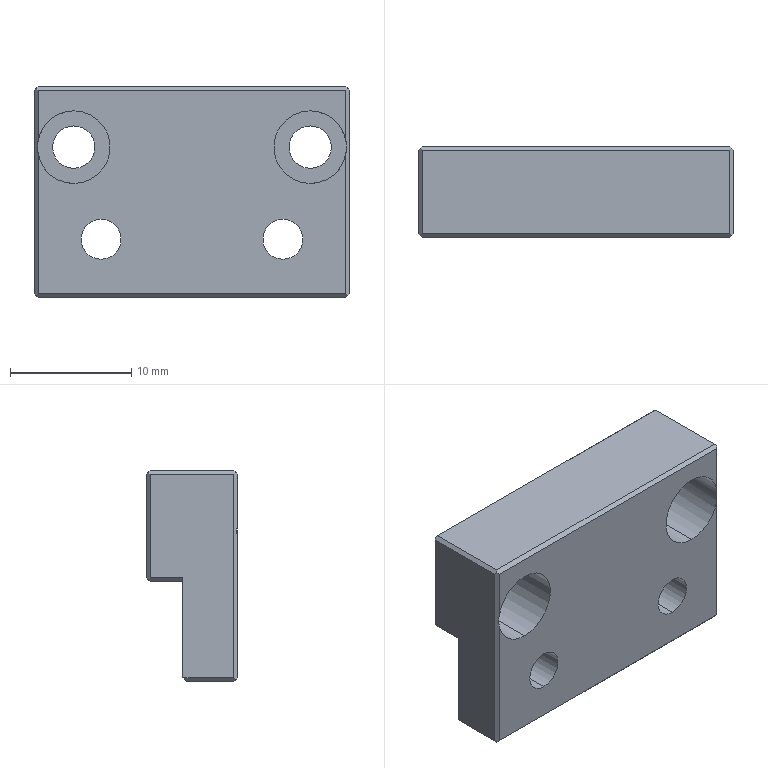Part | NX | 1 solid | 38 faces | box 26 x 7.5 x 17.4 mm | volume 2351 mm3 | plane 26 | cylinder 12 | commonest cylinder face diameters 3.3 x4 3.5 x4 6 x4
STEP:
#1=CARTESIAN_POINT('',(13.59,-63.429,11.253));
#2=VERTEX_POINT('',#1);
#3=CARTESIAN_POINT('',(-11.81,-63.429,11.253));
#4=VERTEX_POINT('',#3);
#5=CARTESIAN_POINT('',(0.8897,-63.429,11.253));
#6=DIRECTION('',(-1.,0.,0.));
#7=VECTOR('',#6,1000.);
#8=LINE('',#5,#7);
#9=EDGE_CURVE('',#2,#4,#8,.T.);
#10=ORIENTED_EDGE('',*,*,#9,.F.);
#11=CARTESIAN_POINT('',(13.59,-66.129,11.253));
#12=VERTEX_POINT('',#11);
#13=CARTESIAN_POINT('',(13.59,-64.629,11.253));
#14=DIRECTION('',(0.,1.,0.));
#15=VECTOR('',#14,1000.);
#16=LINE('',#13,#15);
#17=EDGE_CURVE('',#12,#2,#16,.T.);
#18=ORIENTED_EDGE('',*,*,#17,.F.);
#19=CARTESIAN_POINT('',(-11.81,-66.129,11.253));
#20=VERTEX_POINT('',#19);
#21=CARTESIAN_POINT('',(13.89,-66.129,11.253));
#22=DIRECTION('',(1.,0.,0.));
#23=VECTOR('',#22,1000.);
#24=LINE('',#21,#23);
#25=EDGE_CURVE('',#20,#12,#24,.T.);
#26=ORIENTED_EDGE('',*,*,#25,.F.);
#27=CARTESIAN_POINT('',(-11.81,-64.629,11.253));
#28=DIRECTION('',(0.,-1.,0.));
#29=VECTOR('',#28,1000.);
#30=LINE('',#27,#29);
#31=EDGE_CURVE('',#4,#20,#30,.T.);
#32=ORIENTED_EDGE('',*,*,#31,.F.);
#33=EDGE_LOOP('',(#10,#18,#26,#32));
#34=FACE_BOUND('',#33,.T.);
#35=CARTESIAN_POINT('',(13.89,-66.629,11.253));
#36=DIRECTION('',(0.,0.,-1.));
#37=DIRECTION('',(0.,-1.,0.));
#38=AXIS2_PLACEMENT_3D('',#35,#36,#37);
#39=PLANE('',#38);
#40=ADVANCED_FACE('',(#34),#39,.T.);
#41=CARTESIAN_POINT('',(13.59,-66.129,3.303));
#42=VERTEX_POINT('',#41);
#43=CARTESIAN_POINT('',(-12.11,-66.129,3.303));
#44=VERTEX_POINT('',#43);
#45=CARTESIAN_POINT('',(0.7397,-66.129,3.303));
#46=DIRECTION('',(-1.,0.,0.));
#47=VECTOR('',#46,1000.);
#48=LINE('',#45,#47);
#49=EDGE_CURVE('',#42,#44,#48,.T.);
#50=ORIENTED_EDGE('',*,*,#49,.T.);
#51=CARTESIAN_POINT('',(-12.11,-66.129,11.553));
#52=VERTEX_POINT('',#51);
#53=CARTESIAN_POINT('',(-12.11,-66.129,11.106));
#54=DIRECTION('',(0.,0.,-1.));
#55=VECTOR('',#54,1000.);
#56=LINE('',#53,#55);
#57=EDGE_CURVE('',#52,#44,#56,.T.);
#58=ORIENTED_EDGE('',*,*,#57,.F.);
#59=CARTESIAN_POINT('',(13.89,-66.129,-14.447));
#60=DIRECTION('',(-0.7071,0.,0.7071));
#61=VECTOR('',#60,1000.);
#62=LINE('',#59,#61);
#63=EDGE_CURVE('',#20,#52,#62,.T.);
#64=ORIENTED_EDGE('',*,*,#63,.F.);
#65=ORIENTED_EDGE('',*,*,#25,.T.);
#66=CARTESIAN_POINT('',(13.59,-66.129,11.106));
#67=DIRECTION('',(0.,0.,1.));
#68=VECTOR('',#67,1000.);
#69=LINE('',#66,#68);
#70=EDGE_CURVE('',#42,#12,#69,.T.);
#71=ORIENTED_EDGE('',*,*,#70,.F.);
#72=EDGE_LOOP('',(#50,#58,#64,#65,#71));
#73=FACE_BOUND('',#72,.T.);
#74=CARTESIAN_POINT('',(8.39,-66.129,6.153));
#75=VERTEX_POINT('',#74);
#76=CARTESIAN_POINT('',(8.39,-66.129,9.453));
#77=VERTEX_POINT('',#76);
#78=CARTESIAN_POINT('',(8.39,-66.129,7.803));
#79=DIRECTION('',(0.,-1.,0.));
#80=DIRECTION('',(0.,0.,1.));
#81=AXIS2_PLACEMENT_3D('',#78,#79,#80);
#82=CIRCLE('',#81,1.65);
#83=EDGE_CURVE('',#75,#77,#82,.T.);
#84=ORIENTED_EDGE('',*,*,#83,.T.);
#85=CARTESIAN_POINT('',(8.39,-66.129,7.803));
#86=DIRECTION('',(0.,-1.,0.));
#87=DIRECTION('',(0.,0.,1.));
#88=AXIS2_PLACEMENT_3D('',#85,#86,#87);
#89=CIRCLE('',#88,1.65);
#90=EDGE_CURVE('',#77,#75,#89,.T.);
#91=ORIENTED_EDGE('',*,*,#90,.T.);
#92=EDGE_LOOP('',(#84,#91));
#93=FACE_BOUND('',#92,.T.);
#94=CARTESIAN_POINT('',(-6.61,-66.129,6.153));
#95=VERTEX_POINT('',#94);
#96=CARTESIAN_POINT('',(-6.61,-66.129,9.453));
#97=VERTEX_POINT('',#96);
#98=CARTESIAN_POINT('',(-6.61,-66.129,7.803));
#99=DIRECTION('',(0.,-1.,0.));
#100=DIRECTION('',(0.,0.,1.));
#101=AXIS2_PLACEMENT_3D('',#98,#99,#100);
#102=CIRCLE('',#101,1.65);
#103=EDGE_CURVE('',#95,#97,#102,.T.);
#104=ORIENTED_EDGE('',*,*,#103,.T.);
#105=CARTESIAN_POINT('',(-6.61,-66.129,7.803));
#106=DIRECTION('',(0.,-1.,0.));
#107=DIRECTION('',(0.,0.,1.));
#108=AXIS2_PLACEMENT_3D('',#105,#106,#107);
#109=CIRCLE('',#108,1.65);
#110=EDGE_CURVE('',#97,#95,#109,.T.);
#111=ORIENTED_EDGE('',*,*,#110,.T.);
#112=EDGE_LOOP('',(#104,#111));
#113=FACE_BOUND('',#112,.T.);
#114=CARTESIAN_POINT('',(13.89,-66.129,5.503));
#115=DIRECTION('',(0.,1.,0.));
#116=DIRECTION('',(1.,0.,0.));
#117=AXIS2_PLACEMENT_3D('',#114,#115,#116);
#118=PLANE('',#117);
#119=ADVANCED_FACE('',(#73,#93,#113),#118,.T.);
#120=CARTESIAN_POINT('',(-11.81,-70.329,3.003));
#121=VERTEX_POINT('',#120);
#122=CARTESIAN_POINT('',(-11.81,-66.429,3.003));
#123=VERTEX_POINT('',#122);
#124=CARTESIAN_POINT('',(-11.81,-68.379,3.003));
#125=DIRECTION('',(0.,1.,0.));
#126=VECTOR('',#125,1000.);
#127=LINE('',#124,#126);
#128=EDGE_CURVE('',#121,#123,#127,.T.);
#129=ORIENTED_EDGE('',*,*,#128,.T.);
#130=CARTESIAN_POINT('',(13.59,-66.429,3.003));
#131=VERTEX_POINT('',#130);
#132=CARTESIAN_POINT('',(0.7397,-66.429,3.003));
#133=DIRECTION('',(-1.,0.,0.));
#134=VECTOR('',#133,1000.);
#135=LINE('',#132,#134);
#136=EDGE_CURVE('',#131,#123,#135,.T.);
#137=ORIENTED_EDGE('',*,*,#136,.F.);
#138=CARTESIAN_POINT('',(13.59,-70.329,3.003));
#139=VERTEX_POINT('',#138);
#140=CARTESIAN_POINT('',(13.59,-68.379,3.003));
#141=DIRECTION('',(0.,1.,0.));
#142=VECTOR('',#141,1000.);
#143=LINE('',#140,#142);
#144=EDGE_CURVE('',#139,#131,#143,.T.);
#145=ORIENTED_EDGE('',*,*,#144,.F.);
#146=CARTESIAN_POINT('',(0.7397,-70.329,3.003));
#147=DIRECTION('',(1.,0.,0.));
#148=VECTOR('',#147,1000.);
#149=LINE('',#146,#148);
#150=EDGE_CURVE('',#121,#139,#149,.T.);
#151=ORIENTED_EDGE('',*,*,#150,.F.);
#152=EDGE_LOOP('',(#129,#137,#145,#151));
#153=FACE_BOUND('',#152,.T.);
#154=CARTESIAN_POINT('',(13.89,-70.329,3.003));
#155=DIRECTION('',(0.,0.,-1.));
#156=DIRECTION('',(0.,-1.,0.));
#157=AXIS2_PLACEMENT_3D('',#154,#155,#156);
#158=PLANE('',#157);
#159=ADVANCED_FACE('',(#153),#158,.T.);
#160=CARTESIAN_POINT('',(13.59,-70.629,3.303));
#161=VERTEX_POINT('',#160);
#162=CARTESIAN_POINT('',(13.59,-70.629,14.858));
#163=VERTEX_POINT('',#162);
#164=CARTESIAN_POINT('',(13.59,-70.629,11.106));
#165=DIRECTION('',(0.,0.,1.));
#166=VECTOR('',#165,1000.);
#167=LINE('',#164,#166);
#168=EDGE_CURVE('',#161,#163,#167,.T.);
#169=ORIENTED_EDGE('',*,*,#168,.T.);
#170=CARTESIAN_POINT('',(10.64,-70.629,12.403));
#171=VERTEX_POINT('',#170);
#172=CARTESIAN_POINT('',(10.64,-70.629,15.403));
#173=DIRECTION('',(0.,-1.,0.));
#174=DIRECTION('',(0.,0.,1.));
#175=AXIS2_PLACEMENT_3D('',#172,#173,#174);
#176=CIRCLE('',#175,3.);
#177=EDGE_CURVE('',#171,#163,#176,.T.);
#178=ORIENTED_EDGE('',*,*,#177,.F.);
#179=CARTESIAN_POINT('',(10.64,-70.629,18.403));
#180=VERTEX_POINT('',#179);
#181=CARTESIAN_POINT('',(10.64,-70.629,15.403));
#182=DIRECTION('',(0.,-1.,0.));
#183=DIRECTION('',(0.,0.,1.));
#184=AXIS2_PLACEMENT_3D('',#181,#182,#183);
#185=CIRCLE('',#184,3.);
#186=EDGE_CURVE('',#180,#171,#185,.T.);
#187=ORIENTED_EDGE('',*,*,#186,.F.);
#188=CARTESIAN_POINT('',(13.59,-70.629,15.949));
#189=VERTEX_POINT('',#188);
#190=CARTESIAN_POINT('',(10.64,-70.629,15.403));
#191=DIRECTION('',(0.,-1.,0.));
#192=DIRECTION('',(0.,0.,1.));
#193=AXIS2_PLACEMENT_3D('',#190,#191,#192);
#194=CIRCLE('',#193,3.);
#195=EDGE_CURVE('',#189,#180,#194,.T.);
#196=ORIENTED_EDGE('',*,*,#195,.F.);
#197=CARTESIAN_POINT('',(13.59,-70.629,20.103));
#198=VERTEX_POINT('',#197);
#199=CARTESIAN_POINT('',(13.59,-70.629,11.106));
#200=DIRECTION('',(0.,0.,1.));
#201=VECTOR('',#200,1000.);
#202=LINE('',#199,#201);
#203=EDGE_CURVE('',#189,#198,#202,.T.);
#204=ORIENTED_EDGE('',*,*,#203,.T.);
#205=CARTESIAN_POINT('',(-11.81,-70.629,20.103));
#206=VERTEX_POINT('',#205);
#207=CARTESIAN_POINT('',(0.7397,-70.629,20.103));
#208=DIRECTION('',(-1.,0.,0.));
#209=VECTOR('',#208,1000.);
#210=LINE('',#207,#209);
#211=EDGE_CURVE('',#198,#206,#210,.T.);
#212=ORIENTED_EDGE('',*,*,#211,.T.);
#213=CARTESIAN_POINT('',(-11.81,-70.629,15.949));
#214=VERTEX_POINT('',#213);
#215=CARTESIAN_POINT('',(-11.81,-70.629,11.106));
#216=DIRECTION('',(0.,0.,-1.));
#217=VECTOR('',#216,1000.);
#218=LINE('',#215,#217);
#219=EDGE_CURVE('',#206,#214,#218,.T.);
#220=ORIENTED_EDGE('',*,*,#219,.T.);
#221=CARTESIAN_POINT('',(-8.86,-70.629,18.403));
#222=VERTEX_POINT('',#221);
#223=CARTESIAN_POINT('',(-8.86,-70.629,15.403));
#224=DIRECTION('',(0.,-1.,0.));
#225=DIRECTION('',(0.,0.,1.));
#226=AXIS2_PLACEMENT_3D('',#223,#224,#225);
#227=CIRCLE('',#226,3.);
#228=EDGE_CURVE('',#222,#214,#227,.T.);
#229=ORIENTED_EDGE('',*,*,#228,.F.);
#230=CARTESIAN_POINT('',(-8.86,-70.629,12.403));
#231=VERTEX_POINT('',#230);
#232=CARTESIAN_POINT('',(-8.86,-70.629,15.403));
#233=DIRECTION('',(0.,-1.,0.));
#234=DIRECTION('',(0.,0.,1.));
#235=AXIS2_PLACEMENT_3D('',#232,#233,#234);
#236=CIRCLE('',#235,3.);
#237=EDGE_CURVE('',#231,#222,#236,.T.);
#238=ORIENTED_EDGE('',*,*,#237,.F.);
#239=CARTESIAN_POINT('',(-11.81,-70.629,14.858));
#240=VERTEX_POINT('',#239);
#241=CARTESIAN_POINT('',(-8.86,-70.629,15.403));
#242=DIRECTION('',(0.,-1.,0.));
#243=DIRECTION('',(0.,0.,1.));
#244=AXIS2_PLACEMENT_3D('',#241,#242,#243);
#245=CIRCLE('',#244,3.);
#246=EDGE_CURVE('',#240,#231,#245,.T.);
#247=ORIENTED_EDGE('',*,*,#246,.F.);
#248=CARTESIAN_POINT('',(-11.81,-70.629,3.303));
#249=VERTEX_POINT('',#248);
#250=CARTESIAN_POINT('',(-11.81,-70.629,11.106));
#251=DIRECTION('',(0.,0.,-1.));
#252=VECTOR('',#251,1000.);
#253=LINE('',#250,#252);
#254=EDGE_CURVE('',#240,#249,#253,.T.);
#255=ORIENTED_EDGE('',*,*,#254,.T.);
#256=CARTESIAN_POINT('',(0.7397,-70.629,3.303));
#257=DIRECTION('',(1.,0.,0.));
#258=VECTOR('',#257,1000.);
#259=LINE('',#256,#258);
#260=EDGE_CURVE('',#249,#161,#259,.T.);
#261=ORIENTED_EDGE('',*,*,#260,.T.);
#262=EDGE_LOOP('',(#169,#178,#187,#196,#204,#212,#220,#229,#238,#247,#255,#261));
#263=FACE_BOUND('',#262,.T.);
#264=CARTESIAN_POINT('',(8.39,-70.629,6.153));
#265=VERTEX_POINT('',#264);
#266=CARTESIAN_POINT('',(8.39,-70.629,9.453));
#267=VERTEX_POINT('',#266);
#268=CARTESIAN_POINT('',(8.39,-70.629,7.803));
#269=DIRECTION('',(0.,-1.,0.));
#270=DIRECTION('',(0.,0.,1.));
#271=AXIS2_PLACEMENT_3D('',#268,#269,#270);
#272=CIRCLE('',#271,1.65);
#273=EDGE_CURVE('',#265,#267,#272,.T.);
#274=ORIENTED_EDGE('',*,*,#273,.F.);
#275=CARTESIAN_POINT('',(8.39,-70.629,7.803));
#276=DIRECTION('',(0.,-1.,0.));
#277=DIRECTION('',(0.,0.,1.));
#278=AXIS2_PLACEMENT_3D('',#275,#276,#277);
#279=CIRCLE('',#278,1.65);
#280=EDGE_CURVE('',#267,#265,#279,.T.);
#281=ORIENTED_EDGE('',*,*,#280,.F.);
#282=EDGE_LOOP('',(#274,#281));
#283=FACE_BOUND('',#282,.T.);
#284=CARTESIAN_POINT('',(-6.61,-70.629,6.153));
#285=VERTEX_POINT('',#284);
#286=CARTESIAN_POINT('',(-6.61,-70.629,9.453));
#287=VERTEX_POINT('',#286);
#288=CARTESIAN_POINT('',(-6.61,-70.629,7.803));
#289=DIRECTION('',(0.,-1.,0.));
#290=DIRECTION('',(0.,0.,1.));
#291=AXIS2_PLACEMENT_3D('',#288,#289,#290);
#292=CIRCLE('',#291,1.65);
#293=EDGE_CURVE('',#285,#287,#292,.T.);
#294=ORIENTED_EDGE('',*,*,#293,.F.);
#295=CARTESIAN_POINT('',(-6.61,-70.629,7.803));
#296=DIRECTION('',(0.,-1.,0.));
#297=DIRECTION('',(0.,0.,1.));
#298=AXIS2_PLACEMENT_3D('',#295,#296,#297);
#299=CIRCLE('',#298,1.65);
#300=EDGE_CURVE('',#287,#285,#299,.T.);
#301=ORIENTED_EDGE('',*,*,#300,.F.);
#302=EDGE_LOOP('',(#294,#301));
#303=FACE_BOUND('',#302,.T.);
#304=CARTESIAN_POINT('',(13.89,-70.629,20.403));
#305=DIRECTION('',(0.,-1.,0.));
#306=DIRECTION('',(-1.,0.,0.));
#307=AXIS2_PLACEMENT_3D('',#304,#305,#306);
#308=PLANE('',#307);
#309=ADVANCED_FACE('',(#263,#283,#303),#308,.T.);
#310=CARTESIAN_POINT('',(13.59,-70.329,20.403));
#311=VERTEX_POINT('',#310);
#312=CARTESIAN_POINT('',(-11.81,-70.329,20.403));
#313=VERTEX_POINT('',#312);
#314=CARTESIAN_POINT('',(0.7397,-70.329,20.403));
#315=DIRECTION('',(-1.,0.,0.));
#316=VECTOR('',#315,1000.);
#317=LINE('',#314,#316);
#318=EDGE_CURVE('',#311,#313,#317,.T.);
#319=ORIENTED_EDGE('',*,*,#318,.F.);
#320=CARTESIAN_POINT('',(13.59,-63.429,20.403));
#321=VERTEX_POINT('',#320);
#322=CARTESIAN_POINT('',(13.59,-66.879,20.403));
#323=DIRECTION('',(0.,-1.,0.));
#324=VECTOR('',#323,1000.);
#325=LINE('',#322,#324);
#326=EDGE_CURVE('',#321,#311,#325,.T.);
#327=ORIENTED_EDGE('',*,*,#326,.F.);
#328=CARTESIAN_POINT('',(-11.81,-63.429,20.403));
#329=VERTEX_POINT('',#328);
#330=CARTESIAN_POINT('',(0.8897,-63.429,20.403));
#331=DIRECTION('',(-1.,0.,0.));
#332=VECTOR('',#331,1000.);
#333=LINE('',#330,#332);
#334=EDGE_CURVE('',#321,#329,#333,.T.);
#335=ORIENTED_EDGE('',*,*,#334,.T.);
#336=CARTESIAN_POINT('',(-11.81,-67.029,20.403));
#337=DIRECTION('',(0.,-1.,0.));
#338=VECTOR('',#337,1000.);
#339=LINE('',#336,#338);
#340=EDGE_CURVE('',#329,#313,#339,.T.);
#341=ORIENTED_EDGE('',*,*,#340,.T.);
#342=EDGE_LOOP('',(#319,#327,#335,#341));
#343=FACE_BOUND('',#342,.T.);
#344=CARTESIAN_POINT('',(13.89,-63.129,20.403));
#345=DIRECTION('',(0.,0.,1.));
#346=DIRECTION('',(1.,0.,0.));
#347=AXIS2_PLACEMENT_3D('',#344,#345,#346);
#348=PLANE('',#347);
#349=ADVANCED_FACE('',(#343),#348,.T.);
#350=CARTESIAN_POINT('',(13.59,-63.129,11.553));
#351=VERTEX_POINT('',#350);
#352=CARTESIAN_POINT('',(13.59,-63.129,20.103));
#353=VERTEX_POINT('',#352);
#354=CARTESIAN_POINT('',(13.59,-63.129,15.828));
#355=DIRECTION('',(0.,0.,1.));
#356=VECTOR('',#355,1000.);
#357=LINE('',#354,#356);
#358=EDGE_CURVE('',#351,#353,#357,.T.);
#359=ORIENTED_EDGE('',*,*,#358,.F.);
#360=CARTESIAN_POINT('',(-11.81,-63.129,11.553));
#361=VERTEX_POINT('',#360);
#362=CARTESIAN_POINT('',(0.8897,-63.129,11.553));
#363=DIRECTION('',(-1.,0.,0.));
#364=VECTOR('',#363,1000.);
#365=LINE('',#362,#364);
#366=EDGE_CURVE('',#351,#361,#365,.T.);
#367=ORIENTED_EDGE('',*,*,#366,.T.);
#368=CARTESIAN_POINT('',(-11.81,-63.129,20.103));
#369=VERTEX_POINT('',#368);
#370=CARTESIAN_POINT('',(-11.81,-63.129,15.828));
#371=DIRECTION('',(0.,0.,-1.));
#372=VECTOR('',#371,1000.);
#373=LINE('',#370,#372);
#374=EDGE_CURVE('',#369,#361,#373,.T.);
#375=ORIENTED_EDGE('',*,*,#374,.F.);
#376=CARTESIAN_POINT('',(0.8897,-63.129,20.103));
#377=DIRECTION('',(-1.,0.,0.));
#378=VECTOR('',#377,1000.);
#379=LINE('',#376,#378);
#380=EDGE_CURVE('',#353,#369,#379,.T.);
#381=ORIENTED_EDGE('',*,*,#380,.F.);
#382=EDGE_LOOP('',(#359,#367,#375,#381));
#383=FACE_BOUND('',#382,.T.);
#384=CARTESIAN_POINT('',(10.64,-63.129,13.653));
#385=VERTEX_POINT('',#384);
#386=CARTESIAN_POINT('',(10.64,-63.129,17.153));
#387=VERTEX_POINT('',#386);
#388=CARTESIAN_POINT('',(10.64,-63.129,15.403));
#389=DIRECTION('',(0.,-1.,0.));
#390=DIRECTION('',(0.,0.,1.));
#391=AXIS2_PLACEMENT_3D('',#388,#389,#390);
#392=CIRCLE('',#391,1.75);
#393=EDGE_CURVE('',#385,#387,#392,.T.);
#394=ORIENTED_EDGE('',*,*,#393,.T.);
#395=CARTESIAN_POINT('',(10.64,-63.129,15.403));
#396=DIRECTION('',(0.,-1.,0.));
#397=DIRECTION('',(0.,0.,1.));
#398=AXIS2_PLACEMENT_3D('',#395,#396,#397);
#399=CIRCLE('',#398,1.75);
#400=EDGE_CURVE('',#387,#385,#399,.T.);
#401=ORIENTED_EDGE('',*,*,#400,.T.);
#402=EDGE_LOOP('',(#394,#401));
#403=FACE_BOUND('',#402,.T.);
#404=CARTESIAN_POINT('',(-8.86,-63.129,13.653));
#405=VERTEX_POINT('',#404);
#406=CARTESIAN_POINT('',(-8.86,-63.129,17.153));
#407=VERTEX_POINT('',#406);
#408=CARTESIAN_POINT('',(-8.86,-63.129,15.403));
#409=DIRECTION('',(0.,-1.,0.));
#410=DIRECTION('',(0.,0.,1.));
#411=AXIS2_PLACEMENT_3D('',#408,#409,#410);
#412=CIRCLE('',#411,1.75);
#413=EDGE_CURVE('',#405,#407,#412,.T.);
#414=ORIENTED_EDGE('',*,*,#413,.T.);
#415=CARTESIAN_POINT('',(-8.86,-63.129,15.403));
#416=DIRECTION('',(0.,-1.,0.));
#417=DIRECTION('',(0.,0.,1.));
#418=AXIS2_PLACEMENT_3D('',#415,#416,#417);
#419=CIRCLE('',#418,1.75);
#420=EDGE_CURVE('',#407,#405,#419,.T.);
#421=ORIENTED_EDGE('',*,*,#420,.T.);
#422=EDGE_LOOP('',(#414,#421));
#423=FACE_BOUND('',#422,.T.);
#424=CARTESIAN_POINT('',(13.89,-63.129,11.253));
#425=DIRECTION('',(0.,1.,0.));
#426=DIRECTION('',(1.,0.,0.));
#427=AXIS2_PLACEMENT_3D('',#424,#425,#426);
#428=PLANE('',#427);
#429=ADVANCED_FACE('',(#383,#403,#423),#428,.T.);
#430=ORIENTED_EDGE('',*,*,#228,.T.);
#431=CARTESIAN_POINT('',(-11.81,-70.629,15.949));
#432=CARTESIAN_POINT('',(-11.877,-70.562,15.587));
#433=CARTESIAN_POINT('',(-11.877,-70.562,15.219));
#434=CARTESIAN_POINT('',(-11.81,-70.629,14.858));
#435=(BOUNDED_CURVE()B_SPLINE_CURVE(3,(#431,#432,#433,#434),.UNSPECIFIED.,.F.,.F.)B_SPLINE_CURVE_WITH_KNOTS((4,4),(2.959,3.324),.UNSPECIFIED.)CURVE()GEOMETRIC_REPRESENTATION_ITEM()RATIONAL_B_SPLINE_CURVE((1.,0.9889,0.9889,1.))REPRESENTATION_ITEM(''));
#436=EDGE_CURVE('',#214,#240,#435,.T.);
#437=ORIENTED_EDGE('',*,*,#436,.T.);
#438=ORIENTED_EDGE('',*,*,#246,.T.);
#439=CARTESIAN_POINT('',(-8.86,-66.129,12.403));
#440=VERTEX_POINT('',#439);
#441=CARTESIAN_POINT('',(-8.86,-69.629,12.403));
#442=DIRECTION('',(0.,-1.,0.));
#443=VECTOR('',#442,1000.);
#444=LINE('',#441,#443);
#445=EDGE_CURVE('',#231,#440,#444,.F.);
#446=ORIENTED_EDGE('',*,*,#445,.T.);
#447=CARTESIAN_POINT('',(-8.86,-66.129,18.403));
#448=VERTEX_POINT('',#447);
#449=CARTESIAN_POINT('',(-8.86,-66.129,15.403));
#450=DIRECTION('',(0.,-1.,0.));
#451=DIRECTION('',(0.,0.,1.));
#452=AXIS2_PLACEMENT_3D('',#449,#450,#451);
#453=CIRCLE('',#452,3.);
#454=EDGE_CURVE('',#448,#440,#453,.T.);
#455=ORIENTED_EDGE('',*,*,#454,.F.);
#456=CARTESIAN_POINT('',(-8.86,-69.629,18.403));
#457=DIRECTION('',(0.,-1.,0.));
#458=VECTOR('',#457,1000.);
#459=LINE('',#456,#458);
#460=EDGE_CURVE('',#222,#448,#459,.F.);
#461=ORIENTED_EDGE('',*,*,#460,.F.);
#462=EDGE_LOOP('',(#430,#437,#438,#446,#455,#461));
#463=FACE_BOUND('',#462,.T.);
#464=CARTESIAN_POINT('',(-8.86,-69.629,15.403));
#465=DIRECTION('',(0.,-1.,0.));
#466=DIRECTION('',(0.,0.,1.));
#467=AXIS2_PLACEMENT_3D('',#464,#465,#466);
#468=CYLINDRICAL_SURFACE('',#467,3.);
#469=ADVANCED_FACE('',(#463),#468,.F.);
#470=CARTESIAN_POINT('',(-8.86,-66.129,15.403));
#471=DIRECTION('',(0.,-1.,0.));
#472=DIRECTION('',(0.,0.,1.));
#473=AXIS2_PLACEMENT_3D('',#470,#471,#472);
#474=CIRCLE('',#473,3.);
#475=EDGE_CURVE('',#440,#448,#474,.T.);
#476=ORIENTED_EDGE('',*,*,#475,.T.);
#477=ORIENTED_EDGE('',*,*,#454,.T.);
#478=EDGE_LOOP('',(#476,#477));
#479=FACE_BOUND('',#478,.T.);
#480=CARTESIAN_POINT('',(-8.86,-66.129,13.653));
#481=VERTEX_POINT('',#480);
#482=CARTESIAN_POINT('',(-8.86,-66.129,17.153));
#483=VERTEX_POINT('',#482);
#484=CARTESIAN_POINT('',(-8.86,-66.129,15.403));
#485=DIRECTION('',(0.,-1.,0.));
#486=DIRECTION('',(0.,0.,1.));
#487=AXIS2_PLACEMENT_3D('',#484,#485,#486);
#488=CIRCLE('',#487,1.75);
#489=EDGE_CURVE('',#481,#483,#488,.T.);
#490=ORIENTED_EDGE('',*,*,#489,.F.);
#491=CARTESIAN_POINT('',(-8.86,-66.129,15.403));
#492=DIRECTION('',(0.,-1.,0.));
#493=DIRECTION('',(0.,0.,1.));
#494=AXIS2_PLACEMENT_3D('',#491,#492,#493);
#495=CIRCLE('',#494,1.75);
#496=EDGE_CURVE('',#483,#481,#495,.T.);
#497=ORIENTED_EDGE('',*,*,#496,.F.);
#498=EDGE_LOOP('',(#490,#497));
#499=FACE_BOUND('',#498,.T.);
#500=CARTESIAN_POINT('',(-8.86,-66.129,15.403));
#501=DIRECTION('',(0.,-1.,0.));
#502=DIRECTION('',(-1.,0.,0.));
#503=AXIS2_PLACEMENT_3D('',#500,#501,#502);
#504=PLANE('',#503);
#505=ADVANCED_FACE('',(#479,#499),#504,.T.);
#506=ORIENTED_EDGE('',*,*,#489,.T.);
#507=CARTESIAN_POINT('',(-8.86,-69.629,17.153));
#508=DIRECTION('',(0.,-1.,0.));
#509=VECTOR('',#508,1000.);
#510=LINE('',#507,#509);
#511=EDGE_CURVE('',#483,#407,#510,.F.);
#512=ORIENTED_EDGE('',*,*,#511,.T.);
#513=ORIENTED_EDGE('',*,*,#413,.F.);
#514=CARTESIAN_POINT('',(-8.86,-69.629,13.653));
#515=DIRECTION('',(0.,-1.,0.));
#516=VECTOR('',#515,1000.);
#517=LINE('',#514,#516);
#518=EDGE_CURVE('',#481,#405,#517,.F.);
#519=ORIENTED_EDGE('',*,*,#518,.F.);
#520=EDGE_LOOP('',(#506,#512,#513,#519));
#521=FACE_BOUND('',#520,.T.);
#522=CARTESIAN_POINT('',(-8.86,-69.629,15.403));
#523=DIRECTION('',(0.,-1.,0.));
#524=DIRECTION('',(0.,0.,1.));
#525=AXIS2_PLACEMENT_3D('',#522,#523,#524);
#526=CYLINDRICAL_SURFACE('',#525,1.75);
#527=ADVANCED_FACE('',(#521),#526,.F.);
#528=CARTESIAN_POINT('',(10.64,-66.129,13.653));
#529=VERTEX_POINT('',#528);
#530=CARTESIAN_POINT('',(10.64,-66.129,17.153));
#531=VERTEX_POINT('',#530);
#532=CARTESIAN_POINT('',(10.64,-66.129,15.403));
#533=DIRECTION('',(0.,-1.,0.));
#534=DIRECTION('',(0.,0.,1.));
#535=AXIS2_PLACEMENT_3D('',#532,#533,#534);
#536=CIRCLE('',#535,1.75);
#537=EDGE_CURVE('',#529,#531,#536,.T.);
#538=ORIENTED_EDGE('',*,*,#537,.T.);
#539=CARTESIAN_POINT('',(10.64,-69.629,17.153));
#540=DIRECTION('',(0.,-1.,0.));
#541=VECTOR('',#540,1000.);
#542=LINE('',#539,#541);
#543=EDGE_CURVE('',#531,#387,#542,.F.);
#544=ORIENTED_EDGE('',*,*,#543,.T.);
#545=ORIENTED_EDGE('',*,*,#393,.F.);
#546=CARTESIAN_POINT('',(10.64,-69.629,13.653));
#547=DIRECTION('',(0.,-1.,0.));
#548=VECTOR('',#547,1000.);
#549=LINE('',#546,#548);
#550=EDGE_CURVE('',#529,#385,#549,.F.);
#551=ORIENTED_EDGE('',*,*,#550,.F.);
#552=EDGE_LOOP('',(#538,#544,#545,#551));
#553=FACE_BOUND('',#552,.T.);
#554=CARTESIAN_POINT('',(10.64,-69.629,15.403));
#555=DIRECTION('',(0.,-1.,0.));
#556=DIRECTION('',(0.,0.,1.));
#557=AXIS2_PLACEMENT_3D('',#554,#555,#556);
#558=CYLINDRICAL_SURFACE('',#557,1.75);
#559=ADVANCED_FACE('',(#553),#558,.F.);
#560=CARTESIAN_POINT('',(10.64,-66.129,12.403));
#561=VERTEX_POINT('',#560);
#562=CARTESIAN_POINT('',(10.64,-66.129,18.403));
#563=VERTEX_POINT('',#562);
#564=CARTESIAN_POINT('',(10.64,-66.129,15.403));
#565=DIRECTION('',(0.,-1.,0.));
#566=DIRECTION('',(0.,0.,1.));
#567=AXIS2_PLACEMENT_3D('',#564,#565,#566);
#568=CIRCLE('',#567,3.);
#569=EDGE_CURVE('',#561,#563,#568,.T.);
#570=ORIENTED_EDGE('',*,*,#569,.T.);
#571=CARTESIAN_POINT('',(10.64,-66.129,15.403));
#572=DIRECTION('',(0.,-1.,0.));
#573=DIRECTION('',(0.,0.,1.));
#574=AXIS2_PLACEMENT_3D('',#571,#572,#573);
#575=CIRCLE('',#574,3.);
#576=EDGE_CURVE('',#563,#561,#575,.T.);
#577=ORIENTED_EDGE('',*,*,#576,.T.);
#578=EDGE_LOOP('',(#570,#577));
#579=FACE_BOUND('',#578,.T.);
#580=ORIENTED_EDGE('',*,*,#537,.F.);
#581=CARTESIAN_POINT('',(10.64,-66.129,15.403));
#582=DIRECTION('',(0.,-1.,0.));
#583=DIRECTION('',(0.,0.,1.));
#584=AXIS2_PLACEMENT_3D('',#581,#582,#583);
#585=CIRCLE('',#584,1.75);
#586=EDGE_CURVE('',#531,#529,#585,.T.);
#587=ORIENTED_EDGE('',*,*,#586,.F.);
#588=EDGE_LOOP('',(#580,#587));
#589=FACE_BOUND('',#588,.T.);
#590=CARTESIAN_POINT('',(10.64,-66.129,15.403));
#591=DIRECTION('',(0.,-1.,0.));
#592=DIRECTION('',(-1.,0.,0.));
#593=AXIS2_PLACEMENT_3D('',#590,#591,#592);
#594=PLANE('',#593);
#595=ADVANCED_FACE('',(#579,#589),#594,.T.);
#596=ORIENTED_EDGE('',*,*,#177,.T.);
#597=CARTESIAN_POINT('',(13.59,-70.629,14.858));
#598=CARTESIAN_POINT('',(13.657,-70.562,15.219));
#599=CARTESIAN_POINT('',(13.657,-70.562,15.587));
#600=CARTESIAN_POINT('',(13.59,-70.629,15.949));
#601=(BOUNDED_CURVE()B_SPLINE_CURVE(3,(#597,#598,#599,#600),.UNSPECIFIED.,.F.,.F.)B_SPLINE_CURVE_WITH_KNOTS((4,4),(2.959,3.324),.UNSPECIFIED.)CURVE()GEOMETRIC_REPRESENTATION_ITEM()RATIONAL_B_SPLINE_CURVE((1.,0.9889,0.9889,1.))REPRESENTATION_ITEM(''));
#602=EDGE_CURVE('',#163,#189,#601,.T.);
#603=ORIENTED_EDGE('',*,*,#602,.T.);
#604=ORIENTED_EDGE('',*,*,#195,.T.);
#605=CARTESIAN_POINT('',(10.64,-69.629,18.403));
#606=DIRECTION('',(0.,-1.,0.));
#607=VECTOR('',#606,1000.);
#608=LINE('',#605,#607);
#609=EDGE_CURVE('',#563,#180,#608,.T.);
#610=ORIENTED_EDGE('',*,*,#609,.F.);
#611=ORIENTED_EDGE('',*,*,#569,.F.);
#612=CARTESIAN_POINT('',(10.64,-69.629,12.403));
#613=DIRECTION('',(0.,-1.,0.));
#614=VECTOR('',#613,1000.);
#615=LINE('',#612,#614);
#616=EDGE_CURVE('',#561,#171,#615,.T.);
#617=ORIENTED_EDGE('',*,*,#616,.T.);
#618=EDGE_LOOP('',(#596,#603,#604,#610,#611,#617));
#619=FACE_BOUND('',#618,.T.);
#620=CARTESIAN_POINT('',(10.64,-69.629,15.403));
#621=DIRECTION('',(0.,-1.,0.));
#622=DIRECTION('',(0.,0.,1.));
#623=AXIS2_PLACEMENT_3D('',#620,#621,#622);
#624=CYLINDRICAL_SURFACE('',#623,3.);
#625=ADVANCED_FACE('',(#619),#624,.F.);
#626=ORIENTED_EDGE('',*,*,#273,.T.);
#627=CARTESIAN_POINT('',(8.39,-69.629,9.453));
#628=DIRECTION('',(0.,-1.,0.));
#629=VECTOR('',#628,1000.);
#630=LINE('',#627,#629);
#631=EDGE_CURVE('',#77,#267,#630,.T.);
#632=ORIENTED_EDGE('',*,*,#631,.F.);
#633=ORIENTED_EDGE('',*,*,#83,.F.);
#634=CARTESIAN_POINT('',(8.39,-69.629,6.153));
#635=DIRECTION('',(0.,-1.,0.));
#636=VECTOR('',#635,1000.);
#637=LINE('',#634,#636);
#638=EDGE_CURVE('',#75,#265,#637,.T.);
#639=ORIENTED_EDGE('',*,*,#638,.T.);
#640=EDGE_LOOP('',(#626,#632,#633,#639));
#641=FACE_BOUND('',#640,.T.);
#642=CARTESIAN_POINT('',(8.39,-69.629,7.803));
#643=DIRECTION('',(0.,-1.,0.));
#644=DIRECTION('',(0.,0.,1.));
#645=AXIS2_PLACEMENT_3D('',#642,#643,#644);
#646=CYLINDRICAL_SURFACE('',#645,1.65);
#647=ADVANCED_FACE('',(#641),#646,.F.);
#648=ORIENTED_EDGE('',*,*,#293,.T.);
#649=CARTESIAN_POINT('',(-6.61,-69.629,9.453));
#650=DIRECTION('',(0.,-1.,0.));
#651=VECTOR('',#650,1000.);
#652=LINE('',#649,#651);
#653=EDGE_CURVE('',#97,#287,#652,.T.);
#654=ORIENTED_EDGE('',*,*,#653,.F.);
#655=ORIENTED_EDGE('',*,*,#103,.F.);
#656=CARTESIAN_POINT('',(-6.61,-69.629,6.153));
#657=DIRECTION('',(0.,-1.,0.));
#658=VECTOR('',#657,1000.);
#659=LINE('',#656,#658);
#660=EDGE_CURVE('',#95,#285,#659,.T.);
#661=ORIENTED_EDGE('',*,*,#660,.T.);
#662=EDGE_LOOP('',(#648,#654,#655,#661));
#663=FACE_BOUND('',#662,.T.);
#664=CARTESIAN_POINT('',(-6.61,-69.629,7.803));
#665=DIRECTION('',(0.,-1.,0.));
#666=DIRECTION('',(0.,0.,1.));
#667=AXIS2_PLACEMENT_3D('',#664,#665,#666);
#668=CYLINDRICAL_SURFACE('',#667,1.65);
#669=ADVANCED_FACE('',(#663),#668,.F.);
#670=ORIENTED_EDGE('',*,*,#334,.F.);
#671=CARTESIAN_POINT('',(13.74,-63.279,20.253));
#672=VERTEX_POINT('',#671);
#673=CARTESIAN_POINT('',(22.887,-54.132,11.106));
#674=DIRECTION('',(-0.5774,-0.5774,0.5774));
#675=VECTOR('',#674,1000.);
#676=LINE('',#673,#675);
#677=EDGE_CURVE('',#672,#321,#676,.T.);
#678=ORIENTED_EDGE('',*,*,#677,.F.);
#679=CARTESIAN_POINT('',(4.593,-54.132,11.106));
#680=DIRECTION('',(0.5774,-0.5774,0.5774));
#681=VECTOR('',#680,1000.);
#682=LINE('',#679,#681);
#683=EDGE_CURVE('',#353,#672,#682,.T.);
#684=ORIENTED_EDGE('',*,*,#683,.F.);
#685=ORIENTED_EDGE('',*,*,#380,.T.);
#686=CARTESIAN_POINT('',(-11.96,-63.279,20.253));
#687=VERTEX_POINT('',#686);
#688=CARTESIAN_POINT('',(13.89,-37.429,-5.597));
#689=DIRECTION('',(-0.5774,-0.5774,0.5774));
#690=VECTOR('',#689,1000.);
#691=LINE('',#688,#690);
#692=EDGE_CURVE('',#369,#687,#691,.T.);
#693=ORIENTED_EDGE('',*,*,#692,.T.);
#694=CARTESIAN_POINT('',(13.89,-89.129,46.103));
#695=DIRECTION('',(0.5774,-0.5774,0.5774));
#696=VECTOR('',#695,1000.);
#697=LINE('',#694,#696);
#698=EDGE_CURVE('',#687,#329,#697,.T.);
#699=ORIENTED_EDGE('',*,*,#698,.T.);
#700=EDGE_LOOP('',(#670,#678,#684,#685,#693,#699));
#701=FACE_BOUND('',#700,.T.);
#702=CARTESIAN_POINT('',(0.8897,-63.279,20.253));
#703=DIRECTION('',(0.,0.7071,0.7071));
#704=DIRECTION('',(1.,0.,0.));
#705=AXIS2_PLACEMENT_3D('',#702,#703,#704);
#706=PLANE('',#705);
#707=ADVANCED_FACE('',(#701),#706,.T.);
#708=ORIENTED_EDGE('',*,*,#9,.T.);
#709=CARTESIAN_POINT('',(-11.96,-63.279,11.403));
#710=VERTEX_POINT('',#709);
#711=CARTESIAN_POINT('',(13.89,-89.129,-14.447));
#712=DIRECTION('',(0.5774,-0.5774,-0.5774));
#713=VECTOR('',#712,1000.);
#714=LINE('',#711,#713);
#715=EDGE_CURVE('',#710,#4,#714,.T.);
#716=ORIENTED_EDGE('',*,*,#715,.F.);
#717=CARTESIAN_POINT('',(13.89,-37.429,37.253));
#718=DIRECTION('',(-0.5774,-0.5774,-0.5774));
#719=VECTOR('',#718,1000.);
#720=LINE('',#717,#719);
#721=EDGE_CURVE('',#361,#710,#720,.T.);
#722=ORIENTED_EDGE('',*,*,#721,.F.);
#723=ORIENTED_EDGE('',*,*,#366,.F.);
#724=CARTESIAN_POINT('',(13.74,-63.279,11.403));
#725=VERTEX_POINT('',#724);
#726=CARTESIAN_POINT('',(13.89,-63.429,11.253));
#727=DIRECTION('',(0.5774,-0.5774,-0.5774));
#728=VECTOR('',#727,1000.);
#729=LINE('',#726,#728);
#730=EDGE_CURVE('',#351,#725,#729,.T.);
#731=ORIENTED_EDGE('',*,*,#730,.T.);
#732=CARTESIAN_POINT('',(13.89,-63.129,11.553));
#733=DIRECTION('',(0.5774,0.5774,0.5774));
#734=VECTOR('',#733,1000.);
#735=LINE('',#732,#734);
#736=EDGE_CURVE('',#2,#725,#735,.T.);
#737=ORIENTED_EDGE('',*,*,#736,.F.);
#738=EDGE_LOOP('',(#708,#716,#722,#723,#731,#737));
#739=FACE_BOUND('',#738,.T.);
#740=CARTESIAN_POINT('',(0.8897,-63.279,11.403));
#741=DIRECTION('',(0.,-0.7071,0.7071));
#742=DIRECTION('',(-1.,0.,0.));
#743=AXIS2_PLACEMENT_3D('',#740,#741,#742);
#744=PLANE('',#743);
#745=ADVANCED_FACE('',(#739),#744,.F.);
#746=ORIENTED_EDGE('',*,*,#211,.F.);
#747=CARTESIAN_POINT('',(13.74,-70.479,20.253));
#748=VERTEX_POINT('',#747);
#749=CARTESIAN_POINT('',(4.593,-79.626,11.106));
#750=DIRECTION('',(0.5774,0.5774,0.5774));
#751=VECTOR('',#750,1000.);
#752=LINE('',#749,#751);
#753=EDGE_CURVE('',#198,#748,#752,.T.);
#754=ORIENTED_EDGE('',*,*,#753,.T.);
#755=CARTESIAN_POINT('',(22.887,-79.626,11.106));
#756=DIRECTION('',(-0.5774,0.5774,0.5774));
#757=VECTOR('',#756,1000.);
#758=LINE('',#755,#757);
#759=EDGE_CURVE('',#748,#311,#758,.T.);
#760=ORIENTED_EDGE('',*,*,#759,.T.);
#761=ORIENTED_EDGE('',*,*,#318,.T.);
#762=CARTESIAN_POINT('',(-11.96,-70.479,20.253));
#763=VERTEX_POINT('',#762);
#764=CARTESIAN_POINT('',(13.89,-44.629,46.103));
#765=DIRECTION('',(-0.5774,-0.5774,-0.5774));
#766=VECTOR('',#765,1000.);
#767=LINE('',#764,#766);
#768=EDGE_CURVE('',#313,#763,#767,.T.);
#769=ORIENTED_EDGE('',*,*,#768,.T.);
#770=CARTESIAN_POINT('',(13.89,-96.329,-5.597));
#771=DIRECTION('',(-0.5774,0.5774,0.5774));
#772=VECTOR('',#771,1000.);
#773=LINE('',#770,#772);
#774=EDGE_CURVE('',#206,#763,#773,.T.);
#775=ORIENTED_EDGE('',*,*,#774,.F.);
#776=EDGE_LOOP('',(#746,#754,#760,#761,#769,#775));
#777=FACE_BOUND('',#776,.T.);
#778=CARTESIAN_POINT('',(0.7397,-70.479,20.253));
#779=DIRECTION('',(0.,-0.7071,0.7071));
#780=DIRECTION('',(-1.,0.,0.));
#781=AXIS2_PLACEMENT_3D('',#778,#779,#780);
#782=PLANE('',#781);
#783=ADVANCED_FACE('',(#777),#782,.T.);
#784=ORIENTED_EDGE('',*,*,#150,.T.);
#785=CARTESIAN_POINT('',(13.74,-70.479,3.153));
#786=VERTEX_POINT('',#785);
#787=CARTESIAN_POINT('',(2.951,-59.69,-7.635));
#788=DIRECTION('',(0.5774,-0.5774,0.5774));
#789=VECTOR('',#788,1000.);
#790=LINE('',#787,#789);
#791=EDGE_CURVE('',#139,#786,#790,.T.);
#792=ORIENTED_EDGE('',*,*,#791,.T.);
#793=CARTESIAN_POINT('',(24.528,-59.69,-7.635));
#794=DIRECTION('',(0.5774,0.5774,-0.5774));
#795=VECTOR('',#794,1000.);
#796=LINE('',#793,#795);
#797=EDGE_CURVE('',#161,#786,#796,.T.);
#798=ORIENTED_EDGE('',*,*,#797,.F.);
#799=ORIENTED_EDGE('',*,*,#260,.F.);
#800=CARTESIAN_POINT('',(-11.96,-70.479,3.153));
#801=VERTEX_POINT('',#800);
#802=CARTESIAN_POINT('',(13.89,-96.329,29.003));
#803=DIRECTION('',(-0.5774,0.5774,-0.5774));
#804=VECTOR('',#803,1000.);
#805=LINE('',#802,#804);
#806=EDGE_CURVE('',#249,#801,#805,.T.);
#807=ORIENTED_EDGE('',*,*,#806,.T.);
#808=CARTESIAN_POINT('',(-1.172,-59.69,-7.635));
#809=DIRECTION('',(0.5774,0.5774,-0.5774));
#810=VECTOR('',#809,1000.);
#811=LINE('',#808,#810);
#812=EDGE_CURVE('',#801,#121,#811,.T.);
#813=ORIENTED_EDGE('',*,*,#812,.T.);
#814=EDGE_LOOP('',(#784,#792,#798,#799,#807,#813));
#815=FACE_BOUND('',#814,.T.);
#816=CARTESIAN_POINT('',(0.7397,-70.479,3.153));
#817=DIRECTION('',(0.,0.7071,0.7071));
#818=DIRECTION('',(1.,0.,0.));
#819=AXIS2_PLACEMENT_3D('',#816,#817,#818);
#820=PLANE('',#819);
#821=ADVANCED_FACE('',(#815),#820,.F.);
#822=ORIENTED_EDGE('',*,*,#49,.F.);
#823=CARTESIAN_POINT('',(13.74,-66.279,3.153));
#824=VERTEX_POINT('',#823);
#825=CARTESIAN_POINT('',(13.89,-66.429,3.003));
#826=DIRECTION('',(0.5774,-0.5774,-0.5774));
#827=VECTOR('',#826,1000.);
#828=LINE('',#825,#827);
#829=EDGE_CURVE('',#42,#824,#828,.T.);
#830=ORIENTED_EDGE('',*,*,#829,.T.);
#831=CARTESIAN_POINT('',(13.89,-66.129,3.303));
#832=DIRECTION('',(-0.5774,-0.5774,-0.5774));
#833=VECTOR('',#832,1000.);
#834=LINE('',#831,#833);
#835=EDGE_CURVE('',#824,#131,#834,.T.);
#836=ORIENTED_EDGE('',*,*,#835,.T.);
#837=ORIENTED_EDGE('',*,*,#136,.T.);
#838=CARTESIAN_POINT('',(13.89,-92.129,-22.697));
#839=DIRECTION('',(0.5774,-0.5774,-0.5774));
#840=VECTOR('',#839,1000.);
#841=LINE('',#838,#840);
#842=EDGE_CURVE('',#44,#123,#841,.T.);
#843=ORIENTED_EDGE('',*,*,#842,.F.);
#844=EDGE_LOOP('',(#822,#830,#836,#837,#843));
#845=FACE_BOUND('',#844,.T.);
#846=CARTESIAN_POINT('',(0.7397,-66.279,3.153));
#847=DIRECTION('',(0.,0.7071,-0.7071));
#848=DIRECTION('',(-1.,0.,0.));
#849=AXIS2_PLACEMENT_3D('',#846,#847,#848);
#850=PLANE('',#849);
#851=ADVANCED_FACE('',(#845),#850,.T.);
#852=ORIENTED_EDGE('',*,*,#128,.F.);
#853=ORIENTED_EDGE('',*,*,#812,.F.);
#854=CARTESIAN_POINT('',(-12.11,-70.329,3.303));
#855=VERTEX_POINT('',#854);
#856=CARTESIAN_POINT('',(13.89,-96.329,-22.697));
#857=DIRECTION('',(-0.5774,0.5774,0.5774));
#858=VECTOR('',#857,1000.);
#859=LINE('',#856,#858);
#860=EDGE_CURVE('',#801,#855,#859,.T.);
#861=ORIENTED_EDGE('',*,*,#860,.T.);
#862=CARTESIAN_POINT('',(-12.11,-68.379,3.303));
#863=DIRECTION('',(0.,1.,0.));
#864=VECTOR('',#863,1000.);
#865=LINE('',#862,#864);
#866=EDGE_CURVE('',#855,#44,#865,.T.);
#867=ORIENTED_EDGE('',*,*,#866,.T.);
#868=ORIENTED_EDGE('',*,*,#842,.T.);
#869=EDGE_LOOP('',(#852,#853,#861,#867,#868));
#870=FACE_BOUND('',#869,.T.);
#871=CARTESIAN_POINT('',(-11.96,-68.379,3.153));
#872=DIRECTION('',(-0.7071,0.,-0.7071));
#873=DIRECTION('',(-0.7071,0.,0.7071));
#874=AXIS2_PLACEMENT_3D('',#871,#872,#873);
#875=PLANE('',#874);
#876=ADVANCED_FACE('',(#870),#875,.T.);
#877=ORIENTED_EDGE('',*,*,#631,.T.);
#878=ORIENTED_EDGE('',*,*,#280,.T.);
#879=ORIENTED_EDGE('',*,*,#638,.F.);
#880=ORIENTED_EDGE('',*,*,#90,.F.);
#881=EDGE_LOOP('',(#877,#878,#879,#880));
#882=FACE_BOUND('',#881,.T.);
#883=CARTESIAN_POINT('',(8.39,-69.629,7.803));
#884=DIRECTION('',(0.,-1.,0.));
#885=DIRECTION('',(0.,0.,1.));
#886=AXIS2_PLACEMENT_3D('',#883,#884,#885);
#887=CYLINDRICAL_SURFACE('',#886,1.65);
#888=ADVANCED_FACE('',(#882),#887,.F.);
#889=ORIENTED_EDGE('',*,*,#518,.T.);
#890=ORIENTED_EDGE('',*,*,#420,.F.);
#891=ORIENTED_EDGE('',*,*,#511,.F.);
#892=ORIENTED_EDGE('',*,*,#496,.T.);
#893=EDGE_LOOP('',(#889,#890,#891,#892));
#894=FACE_BOUND('',#893,.T.);
#895=CARTESIAN_POINT('',(-8.86,-69.629,15.403));
#896=DIRECTION('',(0.,-1.,0.));
#897=DIRECTION('',(0.,0.,1.));
#898=AXIS2_PLACEMENT_3D('',#895,#896,#897);
#899=CYLINDRICAL_SURFACE('',#898,1.75);
#900=ADVANCED_FACE('',(#894),#899,.F.);
#901=ORIENTED_EDGE('',*,*,#609,.T.);
#902=ORIENTED_EDGE('',*,*,#186,.T.);
#903=ORIENTED_EDGE('',*,*,#616,.F.);
#904=ORIENTED_EDGE('',*,*,#576,.F.);
#905=EDGE_LOOP('',(#901,#902,#903,#904));
#906=FACE_BOUND('',#905,.T.);
#907=CARTESIAN_POINT('',(10.64,-69.629,15.403));
#908=DIRECTION('',(0.,-1.,0.));
#909=DIRECTION('',(0.,0.,1.));
#910=AXIS2_PLACEMENT_3D('',#907,#908,#909);
#911=CYLINDRICAL_SURFACE('',#910,3.);
#912=ADVANCED_FACE('',(#906),#911,.F.);
#913=ORIENTED_EDGE('',*,*,#550,.T.);
#914=ORIENTED_EDGE('',*,*,#400,.F.);
#915=ORIENTED_EDGE('',*,*,#543,.F.);
#916=ORIENTED_EDGE('',*,*,#586,.T.);
#917=EDGE_LOOP('',(#913,#914,#915,#916));
#918=FACE_BOUND('',#917,.T.);
#919=CARTESIAN_POINT('',(10.64,-69.629,15.403));
#920=DIRECTION('',(0.,-1.,0.));
#921=DIRECTION('',(0.,0.,1.));
#922=AXIS2_PLACEMENT_3D('',#919,#920,#921);
#923=CYLINDRICAL_SURFACE('',#922,1.75);
#924=ADVANCED_FACE('',(#918),#923,.F.);
#925=ORIENTED_EDGE('',*,*,#475,.F.);
#926=ORIENTED_EDGE('',*,*,#445,.F.);
#927=ORIENTED_EDGE('',*,*,#237,.T.);
#928=ORIENTED_EDGE('',*,*,#460,.T.);
#929=EDGE_LOOP('',(#925,#926,#927,#928));
#930=FACE_BOUND('',#929,.T.);
#931=CARTESIAN_POINT('',(-8.86,-69.629,15.403));
#932=DIRECTION('',(0.,-1.,0.));
#933=DIRECTION('',(0.,0.,1.));
#934=AXIS2_PLACEMENT_3D('',#931,#932,#933);
#935=CYLINDRICAL_SURFACE('',#934,3.);
#936=ADVANCED_FACE('',(#930),#935,.F.);
#937=ORIENTED_EDGE('',*,*,#653,.T.);
#938=ORIENTED_EDGE('',*,*,#300,.T.);
#939=ORIENTED_EDGE('',*,*,#660,.F.);
#940=ORIENTED_EDGE('',*,*,#110,.F.);
#941=EDGE_LOOP('',(#937,#938,#939,#940));
#942=FACE_BOUND('',#941,.T.);
#943=CARTESIAN_POINT('',(-6.61,-69.629,7.803));
#944=DIRECTION('',(0.,-1.,0.));
#945=DIRECTION('',(0.,0.,1.));
#946=AXIS2_PLACEMENT_3D('',#943,#944,#945);
#947=CYLINDRICAL_SURFACE('',#946,1.65);
#948=ADVANCED_FACE('',(#942),#947,.F.);
#949=CARTESIAN_POINT('',(-12.11,-70.329,20.103));
#950=VERTEX_POINT('',#949);
#951=CARTESIAN_POINT('',(-12.11,-70.329,11.703));
#952=DIRECTION('',(0.,0.,1.));
#953=VECTOR('',#952,1000.);
#954=LINE('',#951,#953);
#955=EDGE_CURVE('',#855,#950,#954,.T.);
#956=ORIENTED_EDGE('',*,*,#955,.T.);
#957=CARTESIAN_POINT('',(-12.11,-63.429,20.103));
#958=VERTEX_POINT('',#957);
#959=CARTESIAN_POINT('',(-12.11,-67.029,20.103));
#960=DIRECTION('',(0.,-1.,0.));
#961=VECTOR('',#960,1000.);
#962=LINE('',#959,#961);
#963=EDGE_CURVE('',#958,#950,#962,.T.);
#964=ORIENTED_EDGE('',*,*,#963,.F.);
#965=CARTESIAN_POINT('',(-12.11,-63.429,11.553));
#966=VERTEX_POINT('',#965);
#967=CARTESIAN_POINT('',(-12.11,-63.429,15.828));
#968=DIRECTION('',(0.,0.,-1.));
#969=VECTOR('',#968,1000.);
#970=LINE('',#967,#969);
#971=EDGE_CURVE('',#958,#966,#970,.T.);
#972=ORIENTED_EDGE('',*,*,#971,.T.);
#973=CARTESIAN_POINT('',(-12.11,-59.69,11.553));
#974=DIRECTION('',(0.,-1.,0.));
#975=VECTOR('',#974,1000.);
#976=LINE('',#973,#975);
#977=EDGE_CURVE('',#966,#52,#976,.T.);
#978=ORIENTED_EDGE('',*,*,#977,.T.);
#979=ORIENTED_EDGE('',*,*,#57,.T.);
#980=ORIENTED_EDGE('',*,*,#866,.F.);
#981=EDGE_LOOP('',(#956,#964,#972,#978,#979,#980));
#982=FACE_BOUND('',#981,.T.);
#983=CARTESIAN_POINT('',(-12.11,-59.69,11.106));
#984=DIRECTION('',(1.,0.,0.));
#985=DIRECTION('',(0.,-1.,0.));
#986=AXIS2_PLACEMENT_3D('',#983,#984,#985);
#987=PLANE('',#986);
#988=ADVANCED_FACE('',(#982),#987,.F.);
#989=ORIENTED_EDGE('',*,*,#963,.T.);
#990=CARTESIAN_POINT('',(13.89,-96.329,46.103));
#991=DIRECTION('',(0.5774,-0.5774,0.5774));
#992=VECTOR('',#991,1000.);
#993=LINE('',#990,#992);
#994=EDGE_CURVE('',#950,#763,#993,.T.);
#995=ORIENTED_EDGE('',*,*,#994,.T.);
#996=ORIENTED_EDGE('',*,*,#768,.F.);
#997=ORIENTED_EDGE('',*,*,#340,.F.);
#998=ORIENTED_EDGE('',*,*,#698,.F.);
#999=CARTESIAN_POINT('',(13.89,-37.429,46.103));
#1000=DIRECTION('',(0.5774,0.5774,0.5774));
#1001=VECTOR('',#1000,1000.);
#1002=LINE('',#999,#1001);
#1003=EDGE_CURVE('',#958,#687,#1002,.T.);
#1004=ORIENTED_EDGE('',*,*,#1003,.F.);
#1005=EDGE_LOOP('',(#989,#995,#996,#997,#998,#1004));
#1006=FACE_BOUND('',#1005,.T.);
#1007=CARTESIAN_POINT('',(-11.96,-67.029,20.253));
#1008=DIRECTION('',(0.7071,0.,-0.7071));
#1009=DIRECTION('',(0.,-1.,0.));
#1010=AXIS2_PLACEMENT_3D('',#1007,#1008,#1009);
#1011=PLANE('',#1010);
#1012=ADVANCED_FACE('',(#1006),#1011,.F.);
#1013=ORIENTED_EDGE('',*,*,#977,.F.);
#1014=CARTESIAN_POINT('',(13.89,-37.429,-14.447));
#1015=DIRECTION('',(-0.5774,-0.5774,0.5774));
#1016=VECTOR('',#1015,1000.);
#1017=LINE('',#1014,#1016);
#1018=EDGE_CURVE('',#710,#966,#1017,.T.);
#1019=ORIENTED_EDGE('',*,*,#1018,.F.);
#1020=ORIENTED_EDGE('',*,*,#715,.T.);
#1021=ORIENTED_EDGE('',*,*,#31,.T.);
#1022=ORIENTED_EDGE('',*,*,#63,.T.);
#1023=EDGE_LOOP('',(#1013,#1019,#1020,#1021,#1022));
#1024=FACE_BOUND('',#1023,.T.);
#1025=CARTESIAN_POINT('',(-11.96,-64.629,11.403));
#1026=DIRECTION('',(-0.7071,0.,-0.7071));
#1027=DIRECTION('',(-0.7071,0.,0.7071));
#1028=AXIS2_PLACEMENT_3D('',#1025,#1026,#1027);
#1029=PLANE('',#1028);
#1030=ADVANCED_FACE('',(#1024),#1029,.T.);
#1031=ORIENTED_EDGE('',*,*,#971,.F.);
#1032=ORIENTED_EDGE('',*,*,#1003,.T.);
#1033=ORIENTED_EDGE('',*,*,#692,.F.);
#1034=ORIENTED_EDGE('',*,*,#374,.T.);
#1035=ORIENTED_EDGE('',*,*,#721,.T.);
#1036=ORIENTED_EDGE('',*,*,#1018,.T.);
#1037=EDGE_LOOP('',(#1031,#1032,#1033,#1034,#1035,#1036));
#1038=FACE_BOUND('',#1037,.T.);
#1039=CARTESIAN_POINT('',(-11.96,-63.279,15.828));
#1040=DIRECTION('',(-0.7071,0.7071,0.));
#1041=DIRECTION('',(0.,0.,1.));
#1042=AXIS2_PLACEMENT_3D('',#1039,#1040,#1041);
#1043=PLANE('',#1042);
#1044=ADVANCED_FACE('',(#1038),#1043,.T.);
#1045=ORIENTED_EDGE('',*,*,#955,.F.);
#1046=ORIENTED_EDGE('',*,*,#860,.F.);
#1047=ORIENTED_EDGE('',*,*,#806,.F.);
#1048=ORIENTED_EDGE('',*,*,#254,.F.);
#1049=ORIENTED_EDGE('',*,*,#436,.F.);
#1050=ORIENTED_EDGE('',*,*,#219,.F.);
#1051=ORIENTED_EDGE('',*,*,#774,.T.);
#1052=ORIENTED_EDGE('',*,*,#994,.F.);
#1053=EDGE_LOOP('',(#1045,#1046,#1047,#1048,#1049,#1050,#1051,#1052));
#1054=FACE_BOUND('',#1053,.T.);
#1055=CARTESIAN_POINT('',(-11.96,-70.479,11.703));
#1056=DIRECTION('',(-0.7071,-0.7071,0.));
#1057=DIRECTION('',(-0.7071,0.7071,0.));
#1058=AXIS2_PLACEMENT_3D('',#1055,#1056,#1057);
#1059=PLANE('',#1058);
#1060=ADVANCED_FACE('',(#1054),#1059,.T.);
#1061=CARTESIAN_POINT('',(13.89,-70.329,3.303));
#1062=VERTEX_POINT('',#1061);
#1063=CARTESIAN_POINT('',(13.89,-66.429,3.303));
#1064=VERTEX_POINT('',#1063);
#1065=CARTESIAN_POINT('',(13.89,-68.379,3.303));
#1066=DIRECTION('',(0.,1.,0.));
#1067=VECTOR('',#1066,1000.);
#1068=LINE('',#1065,#1067);
#1069=EDGE_CURVE('',#1062,#1064,#1068,.T.);
#1070=ORIENTED_EDGE('',*,*,#1069,.T.);
#1071=CARTESIAN_POINT('',(13.89,-66.429,11.553));
#1072=VERTEX_POINT('',#1071);
#1073=CARTESIAN_POINT('',(13.89,-66.429,11.106));
#1074=DIRECTION('',(0.,0.,1.));
#1075=VECTOR('',#1074,1000.);
#1076=LINE('',#1073,#1075);
#1077=EDGE_CURVE('',#1064,#1072,#1076,.T.);
#1078=ORIENTED_EDGE('',*,*,#1077,.T.);
#1079=CARTESIAN_POINT('',(13.89,-63.429,11.553));
#1080=VERTEX_POINT('',#1079);
#1081=CARTESIAN_POINT('',(13.89,-64.629,11.553));
#1082=DIRECTION('',(0.,1.,0.));
#1083=VECTOR('',#1082,1000.);
#1084=LINE('',#1081,#1083);
#1085=EDGE_CURVE('',#1072,#1080,#1084,.T.);
#1086=ORIENTED_EDGE('',*,*,#1085,.T.);
#1087=CARTESIAN_POINT('',(13.89,-63.429,20.103));
#1088=VERTEX_POINT('',#1087);
#1089=CARTESIAN_POINT('',(13.89,-63.429,15.828));
#1090=DIRECTION('',(0.,0.,1.));
#1091=VECTOR('',#1090,1000.);
#1092=LINE('',#1089,#1091);
#1093=EDGE_CURVE('',#1080,#1088,#1092,.T.);
#1094=ORIENTED_EDGE('',*,*,#1093,.T.);
#1095=CARTESIAN_POINT('',(13.89,-70.329,20.103));
#1096=VERTEX_POINT('',#1095);
#1097=CARTESIAN_POINT('',(13.89,-66.879,20.103));
#1098=DIRECTION('',(0.,-1.,0.));
#1099=VECTOR('',#1098,1000.);
#1100=LINE('',#1097,#1099);
#1101=EDGE_CURVE('',#1088,#1096,#1100,.T.);
#1102=ORIENTED_EDGE('',*,*,#1101,.T.);
#1103=CARTESIAN_POINT('',(13.89,-70.329,11.106));
#1104=DIRECTION('',(0.,0.,-1.));
#1105=VECTOR('',#1104,1000.);
#1106=LINE('',#1103,#1105);
#1107=EDGE_CURVE('',#1096,#1062,#1106,.T.);
#1108=ORIENTED_EDGE('',*,*,#1107,.T.);
#1109=EDGE_LOOP('',(#1070,#1078,#1086,#1094,#1102,#1108));
#1110=FACE_BOUND('',#1109,.T.);
#1111=CARTESIAN_POINT('',(13.89,-59.69,11.106));
#1112=DIRECTION('',(1.,0.,0.));
#1113=DIRECTION('',(0.,-1.,0.));
#1114=AXIS2_PLACEMENT_3D('',#1111,#1112,#1113);
#1115=PLANE('',#1114);
#1116=ADVANCED_FACE('',(#1110),#1115,.T.);
#1117=ORIENTED_EDGE('',*,*,#1085,.F.);
#1118=CARTESIAN_POINT('',(13.443,-65.982,11.106));
#1119=DIRECTION('',(-0.5774,0.5774,-0.5774));
#1120=VECTOR('',#1119,1000.);
#1121=LINE('',#1118,#1120);
#1122=EDGE_CURVE('',#1072,#12,#1121,.T.);
#1123=ORIENTED_EDGE('',*,*,#1122,.T.);
#1124=ORIENTED_EDGE('',*,*,#17,.T.);
#1125=ORIENTED_EDGE('',*,*,#736,.T.);
#1126=CARTESIAN_POINT('',(13.443,-62.982,11.106));
#1127=DIRECTION('',(-0.5774,0.5774,-0.5774));
#1128=VECTOR('',#1127,1000.);
#1129=LINE('',#1126,#1128);
#1130=EDGE_CURVE('',#1080,#725,#1129,.T.);
#1131=ORIENTED_EDGE('',*,*,#1130,.F.);
#1132=EDGE_LOOP('',(#1117,#1123,#1124,#1125,#1131));
#1133=FACE_BOUND('',#1132,.T.);
#1134=CARTESIAN_POINT('',(13.74,-64.629,11.403));
#1135=DIRECTION('',(0.7071,0.,-0.7071));
#1136=DIRECTION('',(0.,-1.,0.));
#1137=AXIS2_PLACEMENT_3D('',#1134,#1135,#1136);
#1138=PLANE('',#1137);
#1139=ADVANCED_FACE('',(#1133),#1138,.T.);
#1140=ORIENTED_EDGE('',*,*,#168,.F.);
#1141=ORIENTED_EDGE('',*,*,#797,.T.);
#1142=CARTESIAN_POINT('',(24.528,-59.69,13.942));
#1143=DIRECTION('',(-0.5774,-0.5774,-0.5774));
#1144=VECTOR('',#1143,1000.);
#1145=LINE('',#1142,#1144);
#1146=EDGE_CURVE('',#1062,#786,#1145,.T.);
#1147=ORIENTED_EDGE('',*,*,#1146,.F.);
#1148=ORIENTED_EDGE('',*,*,#1107,.F.);
#1149=CARTESIAN_POINT('',(22.887,-61.332,11.106));
#1150=DIRECTION('',(-0.5774,-0.5774,0.5774));
#1151=VECTOR('',#1150,1000.);
#1152=LINE('',#1149,#1151);
#1153=EDGE_CURVE('',#1096,#748,#1152,.T.);
#1154=ORIENTED_EDGE('',*,*,#1153,.T.);
#1155=ORIENTED_EDGE('',*,*,#753,.F.);
#1156=ORIENTED_EDGE('',*,*,#203,.F.);
#1157=ORIENTED_EDGE('',*,*,#602,.F.);
#1158=EDGE_LOOP('',(#1140,#1141,#1147,#1148,#1154,#1155,#1156,#1157));
#1159=FACE_BOUND('',#1158,.T.);
#1160=CARTESIAN_POINT('',(13.74,-70.479,11.703));
#1161=DIRECTION('',(0.7071,-0.7071,0.));
#1162=DIRECTION('',(0.,0.,-1.));
#1163=AXIS2_PLACEMENT_3D('',#1160,#1161,#1162);
#1164=PLANE('',#1163);
#1165=ADVANCED_FACE('',(#1159),#1164,.T.);
#1166=ORIENTED_EDGE('',*,*,#1101,.F.);
#1167=CARTESIAN_POINT('',(22.887,-72.426,11.106));
#1168=DIRECTION('',(-0.5774,0.5774,0.5774));
#1169=VECTOR('',#1168,1000.);
#1170=LINE('',#1167,#1169);
#1171=EDGE_CURVE('',#1088,#672,#1170,.T.);
#1172=ORIENTED_EDGE('',*,*,#1171,.T.);
#1173=ORIENTED_EDGE('',*,*,#677,.T.);
#1174=ORIENTED_EDGE('',*,*,#326,.T.);
#1175=ORIENTED_EDGE('',*,*,#759,.F.);
#1176=ORIENTED_EDGE('',*,*,#1153,.F.);
#1177=EDGE_LOOP('',(#1166,#1172,#1173,#1174,#1175,#1176));
#1178=FACE_BOUND('',#1177,.T.);
#1179=CARTESIAN_POINT('',(13.74,-66.879,20.253));
#1180=DIRECTION('',(0.7071,0.,0.7071));
#1181=DIRECTION('',(0.,-1.,0.));
#1182=AXIS2_PLACEMENT_3D('',#1179,#1180,#1181);
#1183=PLANE('',#1182);
#1184=ADVANCED_FACE('',(#1178),#1183,.T.);
#1185=ORIENTED_EDGE('',*,*,#1093,.F.);
#1186=ORIENTED_EDGE('',*,*,#1130,.T.);
#1187=ORIENTED_EDGE('',*,*,#730,.F.);
#1188=ORIENTED_EDGE('',*,*,#358,.T.);
#1189=ORIENTED_EDGE('',*,*,#683,.T.);
#1190=ORIENTED_EDGE('',*,*,#1171,.F.);
#1191=EDGE_LOOP('',(#1185,#1186,#1187,#1188,#1189,#1190));
#1192=FACE_BOUND('',#1191,.T.);
#1193=CARTESIAN_POINT('',(13.74,-63.279,15.828));
#1194=DIRECTION('',(0.7071,0.7071,0.));
#1195=DIRECTION('',(0.,0.,-1.));
#1196=AXIS2_PLACEMENT_3D('',#1193,#1194,#1195);
#1197=PLANE('',#1196);
#1198=ADVANCED_FACE('',(#1192),#1197,.T.);
#1199=ORIENTED_EDGE('',*,*,#1077,.F.);
#1200=CARTESIAN_POINT('',(13.89,-66.429,3.303));
#1201=DIRECTION('',(0.5774,-0.5774,0.5774));
#1202=VECTOR('',#1201,1000.);
#1203=LINE('',#1200,#1202);
#1204=EDGE_CURVE('',#824,#1064,#1203,.T.);
#1205=ORIENTED_EDGE('',*,*,#1204,.F.);
#1206=ORIENTED_EDGE('',*,*,#829,.F.);
#1207=ORIENTED_EDGE('',*,*,#70,.T.);
#1208=ORIENTED_EDGE('',*,*,#1122,.F.);
#1209=EDGE_LOOP('',(#1199,#1205,#1206,#1207,#1208));
#1210=FACE_BOUND('',#1209,.T.);
#1211=CARTESIAN_POINT('',(13.74,-66.279,7.128));
#1212=DIRECTION('',(0.7071,0.7071,0.));
#1213=DIRECTION('',(0.,0.,-1.));
#1214=AXIS2_PLACEMENT_3D('',#1211,#1212,#1213);
#1215=PLANE('',#1214);
#1216=ADVANCED_FACE('',(#1210),#1215,.T.);
#1217=ORIENTED_EDGE('',*,*,#1069,.F.);
#1218=ORIENTED_EDGE('',*,*,#1146,.T.);
#1219=ORIENTED_EDGE('',*,*,#791,.F.);
#1220=ORIENTED_EDGE('',*,*,#144,.T.);
#1221=ORIENTED_EDGE('',*,*,#835,.F.);
#1222=ORIENTED_EDGE('',*,*,#1204,.T.);
#1223=EDGE_LOOP('',(#1217,#1218,#1219,#1220,#1221,#1222));
#1224=FACE_BOUND('',#1223,.T.);
#1225=CARTESIAN_POINT('',(13.74,-68.379,3.153));
#1226=DIRECTION('',(0.7071,0.,-0.7071));
#1227=DIRECTION('',(0.,-1.,0.));
#1228=AXIS2_PLACEMENT_3D('',#1225,#1226,#1227);
#1229=PLANE('',#1228);
#1230=ADVANCED_FACE('',(#1224),#1229,.T.);
#1231=CLOSED_SHELL('',(#40,#119,#159,#309,#349,#429,#469,#505,#527,#559,#595,#625,#647,#669,#707,#745,#783,#821,#851,#876,#888,#900,#912,#924,#936,#948,#988,#1012,#1030,#1044,#1060,#1116,#1139,#1165,#1184,#1198,#1216,#1230));
#1232=MANIFOLD_SOLID_BREP('',#1231);
#1233=(LENGTH_UNIT()NAMED_UNIT(*)SI_UNIT(.MILLI.,.METRE.));
#1234=UNCERTAINTY_MEASURE_WITH_UNIT(LENGTH_MEASURE(0.00001),#1233,'','');
#1235=(NAMED_UNIT(*)PLANE_ANGLE_UNIT()SI_UNIT($,.RADIAN.));
#1236=(NAMED_UNIT(*)SI_UNIT($,.STERADIAN.)SOLID_ANGLE_UNIT());
#1237=(GEOMETRIC_REPRESENTATION_CONTEXT(3)GLOBAL_UNCERTAINTY_ASSIGNED_CONTEXT((#1234))GLOBAL_UNIT_ASSIGNED_CONTEXT((#1233,#1235,#1236))REPRESENTATION_CONTEXT('',''));
#1238=ADVANCED_BREP_SHAPE_REPRESENTATION('',(#1232),#1237);